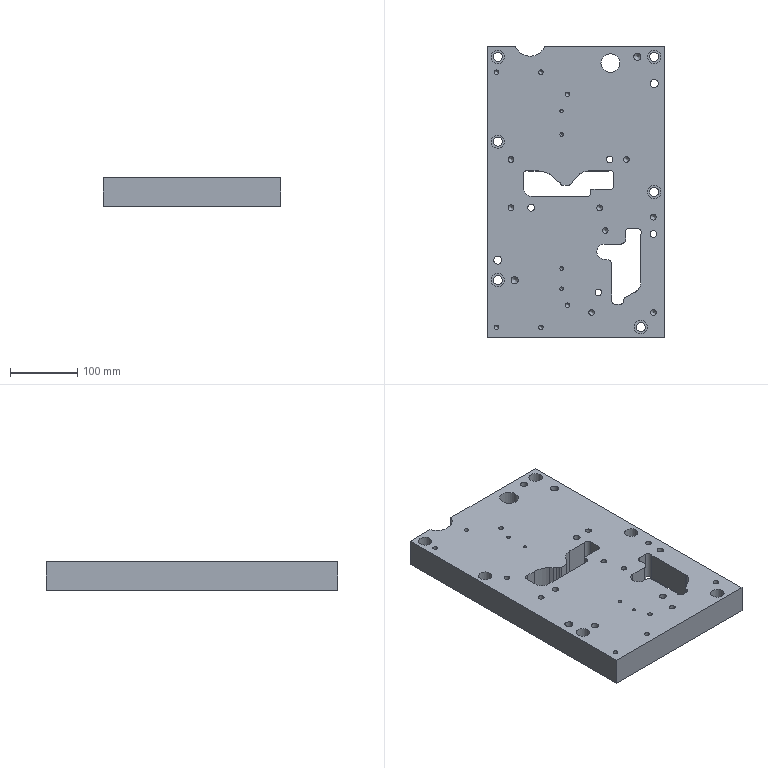Part | STEP file | lll_id726_x_t | 1 solid | 131 faces | box 265 x 435 x 42 mm | volume 4332520 mm3 | cylinder 78 | plane 33 | cone 20 | commonest cylinder face diameters 1 x8 8.506 x8 11 x8 6.806 x6 13.509 x6 20.008 x6